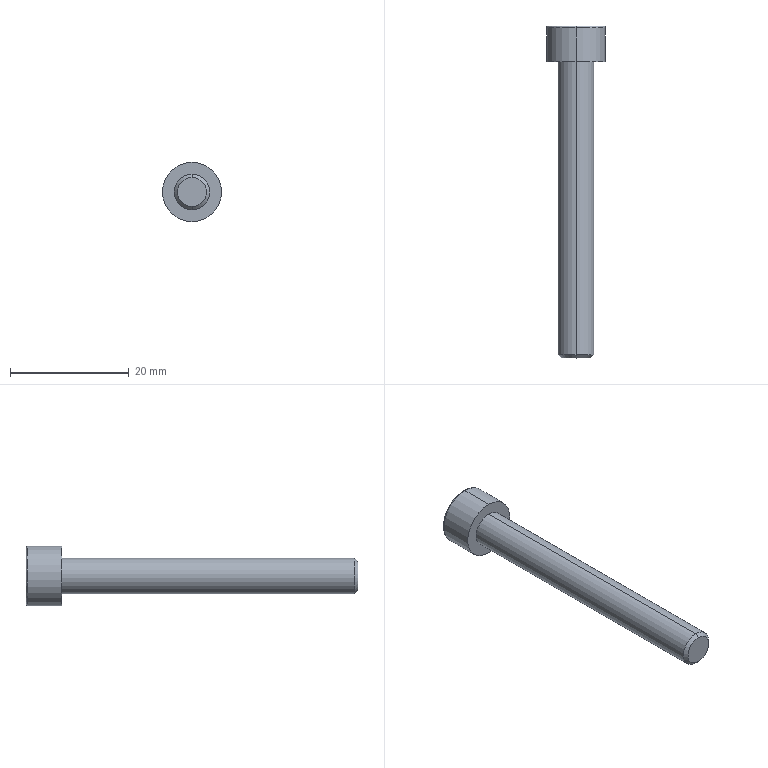Part | SolidWorks | features BaseBody 1 | 1 solid | 18 faces | box 10 x 56 x 10 mm | volume 1815 mm3 | plane 10 | cylinder 4 | cone 2 | torus 2 | commonest cylinder face diameters 6 x2 10 x2
STEP:
#1=CARTESIAN_POINT('',(0.,-50.,-2.445));
#2=VERTEX_POINT('',#1);
#3=CARTESIAN_POINT('',(0.,-50.,2.445));
#4=VERTEX_POINT('',#3);
#5=CARTESIAN_POINT('',(0.,-50.,0.));
#6=DIRECTION('',(0.,-1.,0.));
#7=DIRECTION('',(0.,0.,-1.));
#8=AXIS2_PLACEMENT_3D('',#5,#6,#7);
#9=CIRCLE('',#8,2.445);
#10=EDGE_CURVE('',#2,#4,#9,.T.);
#11=ORIENTED_EDGE('',*,*,#10,.F.);
#12=CARTESIAN_POINT('',(0.,-49.445,-3.));
#13=VERTEX_POINT('',#12);
#14=CARTESIAN_POINT('',(0.,-50.,-2.445));
#15=DIRECTION('',(0.,0.7071,-0.7071));
#16=VECTOR('',#15,1000.);
#17=LINE('',#14,#16);
#18=EDGE_CURVE('',#2,#13,#17,.T.);
#19=ORIENTED_EDGE('',*,*,#18,.T.);
#20=CARTESIAN_POINT('',(0.,-49.445,3.));
#21=VERTEX_POINT('',#20);
#22=CARTESIAN_POINT('',(0.,-49.445,0.));
#23=DIRECTION('',(0.,1.,0.));
#24=DIRECTION('',(0.,0.,-1.));
#25=AXIS2_PLACEMENT_3D('',#22,#23,#24);
#26=CIRCLE('',#25,3.);
#27=EDGE_CURVE('',#21,#13,#26,.T.);
#28=ORIENTED_EDGE('',*,*,#27,.F.);
#29=CARTESIAN_POINT('',(0.,-50.,2.445));
#30=DIRECTION('',(0.,0.7071,0.7071));
#31=VECTOR('',#30,1000.);
#32=LINE('',#29,#31);
#33=EDGE_CURVE('',#4,#21,#32,.T.);
#34=ORIENTED_EDGE('',*,*,#33,.F.);
#35=EDGE_LOOP('',(#11,#19,#28,#34));
#36=FACE_OUTER_BOUND('',#35,.T.);
#37=CARTESIAN_POINT('',(0.,-50.,0.));
#38=DIRECTION('',(0.,1.,0.));
#39=DIRECTION('',(0.,0.,1.));
#40=AXIS2_PLACEMENT_3D('',#37,#38,#39);
#41=CONICAL_SURFACE('',#40,2.445,0.7854);
#42=ADVANCED_FACE('',(#36),#41,.T.);
#43=ORIENTED_EDGE('',*,*,#27,.T.);
#44=CARTESIAN_POINT('',(0.,0.,-3.));
#45=VERTEX_POINT('',#44);
#46=CARTESIAN_POINT('',(0.,-50.,-3.));
#47=DIRECTION('',(0.,1.,0.));
#48=VECTOR('',#47,1000.);
#49=LINE('',#46,#48);
#50=EDGE_CURVE('',#13,#45,#49,.T.);
#51=ORIENTED_EDGE('',*,*,#50,.T.);
#52=CARTESIAN_POINT('',(0.,0.,3.));
#53=VERTEX_POINT('',#52);
#54=CARTESIAN_POINT('',(0.,0.,0.));
#55=DIRECTION('',(0.,-1.,0.));
#56=DIRECTION('',(0.,0.,1.));
#57=AXIS2_PLACEMENT_3D('',#54,#55,#56);
#58=CIRCLE('',#57,3.);
#59=EDGE_CURVE('',#45,#53,#58,.T.);
#60=ORIENTED_EDGE('',*,*,#59,.T.);
#61=CARTESIAN_POINT('',(0.,-50.,3.));
#62=DIRECTION('',(0.,1.,0.));
#63=VECTOR('',#62,1000.);
#64=LINE('',#61,#63);
#65=EDGE_CURVE('',#21,#53,#64,.T.);
#66=ORIENTED_EDGE('',*,*,#65,.F.);
#67=EDGE_LOOP('',(#43,#51,#60,#66));
#68=FACE_OUTER_BOUND('',#67,.T.);
#69=CARTESIAN_POINT('',(0.,-50.,0.));
#70=DIRECTION('',(0.,1.,0.));
#71=DIRECTION('',(0.,0.,1.));
#72=AXIS2_PLACEMENT_3D('',#69,#70,#71);
#73=CYLINDRICAL_SURFACE('',#72,3.);
#74=ADVANCED_FACE('',(#68),#73,.T.);
#75=CARTESIAN_POINT('',(0.,5.7,-5.));
#76=VERTEX_POINT('',#75);
#77=CARTESIAN_POINT('',(0.,5.7,5.));
#78=VERTEX_POINT('',#77);
#79=CARTESIAN_POINT('',(0.,5.7,0.));
#80=DIRECTION('',(0.,-1.,0.));
#81=DIRECTION('',(0.,0.,1.));
#82=AXIS2_PLACEMENT_3D('',#79,#80,#81);
#83=CIRCLE('',#82,5.);
#84=EDGE_CURVE('',#76,#78,#83,.T.);
#85=ORIENTED_EDGE('',*,*,#84,.F.);
#86=CARTESIAN_POINT('',(0.,6.,-4.7));
#87=VERTEX_POINT('',#86);
#88=CARTESIAN_POINT('',(0.,5.7,-4.7));
#89=DIRECTION('',(1.,0.,0.));
#90=DIRECTION('',(0.,0.,-1.));
#91=AXIS2_PLACEMENT_3D('',#88,#89,#90);
#92=CIRCLE('',#91,0.3);
#93=EDGE_CURVE('',#76,#87,#92,.T.);
#94=ORIENTED_EDGE('',*,*,#93,.T.);
#95=CARTESIAN_POINT('',(0.,6.,4.7));
#96=VERTEX_POINT('',#95);
#97=CARTESIAN_POINT('',(0.,6.,0.));
#98=DIRECTION('',(0.,1.,0.));
#99=DIRECTION('',(0.,0.,1.));
#100=AXIS2_PLACEMENT_3D('',#97,#98,#99);
#101=CIRCLE('',#100,4.7);
#102=EDGE_CURVE('',#96,#87,#101,.T.);
#103=ORIENTED_EDGE('',*,*,#102,.F.);
#104=CARTESIAN_POINT('',(0.,5.7,4.7));
#105=DIRECTION('',(-1.,0.,0.));
#106=DIRECTION('',(0.,0.,1.));
#107=AXIS2_PLACEMENT_3D('',#104,#105,#106);
#108=CIRCLE('',#107,0.3);
#109=EDGE_CURVE('',#78,#96,#108,.T.);
#110=ORIENTED_EDGE('',*,*,#109,.F.);
#111=EDGE_LOOP('',(#85,#94,#103,#110));
#112=FACE_OUTER_BOUND('',#111,.T.);
#113=CARTESIAN_POINT('',(0.,5.7,0.));
#114=DIRECTION('',(0.,1.,0.));
#115=DIRECTION('',(0.,0.,1.));
#116=AXIS2_PLACEMENT_3D('',#113,#114,#115);
#117=TOROIDAL_SURFACE('',#116,4.7,0.3);
#118=ADVANCED_FACE('',(#112),#117,.T.);
#119=ORIENTED_EDGE('',*,*,#84,.T.);
#120=CARTESIAN_POINT('',(0.,0.,5.));
#121=VERTEX_POINT('',#120);
#122=CARTESIAN_POINT('',(0.,6.,5.));
#123=DIRECTION('',(0.,-1.,0.));
#124=VECTOR('',#123,1000.);
#125=LINE('',#122,#124);
#126=EDGE_CURVE('',#78,#121,#125,.T.);
#127=ORIENTED_EDGE('',*,*,#126,.T.);
#128=CARTESIAN_POINT('',(0.,0.,-5.));
#129=VERTEX_POINT('',#128);
#130=CARTESIAN_POINT('',(0.,0.,0.));
#131=DIRECTION('',(0.,1.,0.));
#132=DIRECTION('',(0.,0.,1.));
#133=AXIS2_PLACEMENT_3D('',#130,#131,#132);
#134=CIRCLE('',#133,5.);
#135=EDGE_CURVE('',#121,#129,#134,.T.);
#136=ORIENTED_EDGE('',*,*,#135,.T.);
#137=CARTESIAN_POINT('',(0.,6.,-5.));
#138=DIRECTION('',(0.,-1.,0.));
#139=VECTOR('',#138,1000.);
#140=LINE('',#137,#139);
#141=EDGE_CURVE('',#76,#129,#140,.T.);
#142=ORIENTED_EDGE('',*,*,#141,.F.);
#143=EDGE_LOOP('',(#119,#127,#136,#142));
#144=FACE_OUTER_BOUND('',#143,.T.);
#145=CARTESIAN_POINT('',(0.,6.,0.));
#146=DIRECTION('',(0.,-1.,0.));
#147=DIRECTION('',(0.,0.,-1.));
#148=AXIS2_PLACEMENT_3D('',#145,#146,#147);
#149=CYLINDRICAL_SURFACE('',#148,5.);
#150=ADVANCED_FACE('',(#144),#149,.T.);
#151=CARTESIAN_POINT('',(0.,-50.,0.));
#152=DIRECTION('',(0.,-1.,0.));
#153=DIRECTION('',(0.,0.,-1.));
#154=AXIS2_PLACEMENT_3D('',#151,#152,#153);
#155=CIRCLE('',#154,2.445);
#156=EDGE_CURVE('',#4,#2,#155,.T.);
#157=ORIENTED_EDGE('',*,*,#156,.T.);
#158=ORIENTED_EDGE('',*,*,#10,.T.);
#159=EDGE_LOOP('',(#157,#158));
#160=FACE_OUTER_BOUND('',#159,.T.);
#161=CARTESIAN_POINT('',(0.,-50.,0.));
#162=DIRECTION('',(0.,-1.,0.));
#163=DIRECTION('',(0.,0.,-1.));
#164=AXIS2_PLACEMENT_3D('',#161,#162,#163);
#165=PLANE('',#164);
#166=ADVANCED_FACE('',(#160),#165,.T.);
#167=CARTESIAN_POINT('',(1.466,3.,2.54));
#168=VERTEX_POINT('',#167);
#169=CARTESIAN_POINT('',(2.933,3.,0.));
#170=VERTEX_POINT('',#169);
#171=CARTESIAN_POINT('',(1.466,3.,2.54));
#172=DIRECTION('',(0.5,0.,-0.866));
#173=VECTOR('',#172,1000.);
#174=LINE('',#171,#173);
#175=EDGE_CURVE('',#168,#170,#174,.T.);
#176=ORIENTED_EDGE('',*,*,#175,.T.);
#177=CARTESIAN_POINT('',(1.466,3.,-2.54));
#178=VERTEX_POINT('',#177);
#179=CARTESIAN_POINT('',(2.933,3.,0.));
#180=DIRECTION('',(-0.5,0.,-0.866));
#181=VECTOR('',#180,1000.);
#182=LINE('',#179,#181);
#183=EDGE_CURVE('',#170,#178,#182,.T.);
#184=ORIENTED_EDGE('',*,*,#183,.T.);
#185=CARTESIAN_POINT('',(-1.466,3.,-2.54));
#186=VERTEX_POINT('',#185);
#187=CARTESIAN_POINT('',(1.466,3.,-2.54));
#188=DIRECTION('',(-1.,0.,0.));
#189=VECTOR('',#188,1000.);
#190=LINE('',#187,#189);
#191=EDGE_CURVE('',#178,#186,#190,.T.);
#192=ORIENTED_EDGE('',*,*,#191,.T.);
#193=CARTESIAN_POINT('',(-2.933,3.,0.));
#194=VERTEX_POINT('',#193);
#195=CARTESIAN_POINT('',(-1.466,3.,-2.54));
#196=DIRECTION('',(-0.5,0.,0.866));
#197=VECTOR('',#196,1000.);
#198=LINE('',#195,#197);
#199=EDGE_CURVE('',#186,#194,#198,.T.);
#200=ORIENTED_EDGE('',*,*,#199,.T.);
#201=CARTESIAN_POINT('',(-1.466,3.,2.54));
#202=VERTEX_POINT('',#201);
#203=CARTESIAN_POINT('',(-2.933,3.,0.));
#204=DIRECTION('',(0.5,0.,0.866));
#205=VECTOR('',#204,1000.);
#206=LINE('',#203,#205);
#207=EDGE_CURVE('',#194,#202,#206,.T.);
#208=ORIENTED_EDGE('',*,*,#207,.T.);
#209=CARTESIAN_POINT('',(-1.466,3.,2.54));
#210=DIRECTION('',(1.,0.,0.));
#211=VECTOR('',#210,1000.);
#212=LINE('',#209,#211);
#213=EDGE_CURVE('',#202,#168,#212,.T.);
#214=ORIENTED_EDGE('',*,*,#213,.T.);
#215=EDGE_LOOP('',(#176,#184,#192,#200,#208,#214));
#216=FACE_OUTER_BOUND('',#215,.T.);
#217=CARTESIAN_POINT('',(0.,3.,0.));
#218=DIRECTION('',(0.,1.,0.));
#219=DIRECTION('',(1.,0.,0.));
#220=AXIS2_PLACEMENT_3D('',#217,#218,#219);
#221=PLANE('',#220);
#222=ADVANCED_FACE('',(#216),#221,.T.);
#223=CARTESIAN_POINT('',(2.933,6.,0.));
#224=VERTEX_POINT('',#223);
#225=CARTESIAN_POINT('',(1.466,6.,-2.54));
#226=VERTEX_POINT('',#225);
#227=CARTESIAN_POINT('',(2.933,6.,0.));
#228=DIRECTION('',(-0.5,0.,-0.866));
#229=VECTOR('',#228,1000.);
#230=LINE('',#227,#229);
#231=EDGE_CURVE('',#224,#226,#230,.T.);
#232=ORIENTED_EDGE('',*,*,#231,.T.);
#233=CARTESIAN_POINT('',(1.466,3.,-2.54));
#234=DIRECTION('',(0.,1.,0.));
#235=VECTOR('',#234,1000.);
#236=LINE('',#233,#235);
#237=EDGE_CURVE('',#178,#226,#236,.T.);
#238=ORIENTED_EDGE('',*,*,#237,.F.);
#239=ORIENTED_EDGE('',*,*,#183,.F.);
#240=CARTESIAN_POINT('',(2.933,3.,0.));
#241=DIRECTION('',(0.,1.,0.));
#242=VECTOR('',#241,1000.);
#243=LINE('',#240,#242);
#244=EDGE_CURVE('',#170,#224,#243,.T.);
#245=ORIENTED_EDGE('',*,*,#244,.T.);
#246=EDGE_LOOP('',(#232,#238,#239,#245));
#247=FACE_OUTER_BOUND('',#246,.T.);
#248=CARTESIAN_POINT('',(2.933,3.,0.));
#249=DIRECTION('',(0.866,0.,-0.5));
#250=DIRECTION('',(0.,-1.,0.));
#251=AXIS2_PLACEMENT_3D('',#248,#249,#250);
#252=PLANE('',#251);
#253=ADVANCED_FACE('',(#247),#252,.F.);
#254=CARTESIAN_POINT('',(-1.466,6.,-2.54));
#255=VERTEX_POINT('',#254);
#256=CARTESIAN_POINT('',(1.466,6.,-2.54));
#257=DIRECTION('',(-1.,0.,0.));
#258=VECTOR('',#257,1000.);
#259=LINE('',#256,#258);
#260=EDGE_CURVE('',#226,#255,#259,.T.);
#261=ORIENTED_EDGE('',*,*,#260,.T.);
#262=CARTESIAN_POINT('',(-1.466,3.,-2.54));
#263=DIRECTION('',(0.,1.,0.));
#264=VECTOR('',#263,1000.);
#265=LINE('',#262,#264);
#266=EDGE_CURVE('',#186,#255,#265,.T.);
#267=ORIENTED_EDGE('',*,*,#266,.F.);
#268=ORIENTED_EDGE('',*,*,#191,.F.);
#269=ORIENTED_EDGE('',*,*,#237,.T.);
#270=EDGE_LOOP('',(#261,#267,#268,#269));
#271=FACE_OUTER_BOUND('',#270,.T.);
#272=CARTESIAN_POINT('',(1.466,3.,-2.54));
#273=DIRECTION('',(0.,0.,-1.));
#274=DIRECTION('',(0.,-1.,0.));
#275=AXIS2_PLACEMENT_3D('',#272,#273,#274);
#276=PLANE('',#275);
#277=ADVANCED_FACE('',(#271),#276,.F.);
#278=CARTESIAN_POINT('',(-2.933,6.,0.));
#279=VERTEX_POINT('',#278);
#280=CARTESIAN_POINT('',(-1.466,6.,-2.54));
#281=DIRECTION('',(-0.5,0.,0.866));
#282=VECTOR('',#281,1000.);
#283=LINE('',#280,#282);
#284=EDGE_CURVE('',#255,#279,#283,.T.);
#285=ORIENTED_EDGE('',*,*,#284,.T.);
#286=CARTESIAN_POINT('',(-2.933,3.,0.));
#287=DIRECTION('',(0.,1.,0.));
#288=VECTOR('',#287,1000.);
#289=LINE('',#286,#288);
#290=EDGE_CURVE('',#194,#279,#289,.T.);
#291=ORIENTED_EDGE('',*,*,#290,.F.);
#292=ORIENTED_EDGE('',*,*,#199,.F.);
#293=ORIENTED_EDGE('',*,*,#266,.T.);
#294=EDGE_LOOP('',(#285,#291,#292,#293));
#295=FACE_OUTER_BOUND('',#294,.T.);
#296=CARTESIAN_POINT('',(-1.466,3.,-2.54));
#297=DIRECTION('',(-0.866,0.,-0.5));
#298=DIRECTION('',(-0.5,0.,0.866));
#299=AXIS2_PLACEMENT_3D('',#296,#297,#298);
#300=PLANE('',#299);
#301=ADVANCED_FACE('',(#295),#300,.F.);
#302=CARTESIAN_POINT('',(-1.466,6.,2.54));
#303=VERTEX_POINT('',#302);
#304=CARTESIAN_POINT('',(-2.933,6.,0.));
#305=DIRECTION('',(0.5,0.,0.866));
#306=VECTOR('',#305,1000.);
#307=LINE('',#304,#306);
#308=EDGE_CURVE('',#279,#303,#307,.T.);
#309=ORIENTED_EDGE('',*,*,#308,.T.);
#310=CARTESIAN_POINT('',(-1.466,3.,2.54));
#311=DIRECTION('',(0.,1.,0.));
#312=VECTOR('',#311,1000.);
#313=LINE('',#310,#312);
#314=EDGE_CURVE('',#202,#303,#313,.T.);
#315=ORIENTED_EDGE('',*,*,#314,.F.);
#316=ORIENTED_EDGE('',*,*,#207,.F.);
#317=ORIENTED_EDGE('',*,*,#290,.T.);
#318=EDGE_LOOP('',(#309,#315,#316,#317));
#319=FACE_OUTER_BOUND('',#318,.T.);
#320=CARTESIAN_POINT('',(-2.933,3.,0.));
#321=DIRECTION('',(-0.866,0.,0.5));
#322=DIRECTION('',(0.,1.,0.));
#323=AXIS2_PLACEMENT_3D('',#320,#321,#322);
#324=PLANE('',#323);
#325=ADVANCED_FACE('',(#319),#324,.F.);
#326=CARTESIAN_POINT('',(1.466,6.,2.54));
#327=VERTEX_POINT('',#326);
#328=CARTESIAN_POINT('',(-1.466,6.,2.54));
#329=DIRECTION('',(1.,0.,0.));
#330=VECTOR('',#329,1000.);
#331=LINE('',#328,#330);
#332=EDGE_CURVE('',#303,#327,#331,.T.);
#333=ORIENTED_EDGE('',*,*,#332,.T.);
#334=CARTESIAN_POINT('',(1.466,3.,2.54));
#335=DIRECTION('',(0.,1.,0.));
#336=VECTOR('',#335,1000.);
#337=LINE('',#334,#336);
#338=EDGE_CURVE('',#168,#327,#337,.T.);
#339=ORIENTED_EDGE('',*,*,#338,.F.);
#340=ORIENTED_EDGE('',*,*,#213,.F.);
#341=ORIENTED_EDGE('',*,*,#314,.T.);
#342=EDGE_LOOP('',(#333,#339,#340,#341));
#343=FACE_OUTER_BOUND('',#342,.T.);
#344=CARTESIAN_POINT('',(-1.466,3.,2.54));
#345=DIRECTION('',(0.,0.,1.));
#346=DIRECTION('',(1.,0.,0.));
#347=AXIS2_PLACEMENT_3D('',#344,#345,#346);
#348=PLANE('',#347);
#349=ADVANCED_FACE('',(#343),#348,.F.);
#350=CARTESIAN_POINT('',(1.466,6.,2.54));
#351=DIRECTION('',(0.5,0.,-0.866));
#352=VECTOR('',#351,1000.);
#353=LINE('',#350,#352);
#354=EDGE_CURVE('',#327,#224,#353,.T.);
#355=ORIENTED_EDGE('',*,*,#354,.T.);
#356=ORIENTED_EDGE('',*,*,#244,.F.);
#357=ORIENTED_EDGE('',*,*,#175,.F.);
#358=ORIENTED_EDGE('',*,*,#338,.T.);
#359=EDGE_LOOP('',(#355,#356,#357,#358));
#360=FACE_OUTER_BOUND('',#359,.T.);
#361=CARTESIAN_POINT('',(1.466,3.,2.54));
#362=DIRECTION('',(0.866,0.,0.5));
#363=DIRECTION('',(0.,-1.,0.));
#364=AXIS2_PLACEMENT_3D('',#361,#362,#363);
#365=PLANE('',#364);
#366=ADVANCED_FACE('',(#360),#365,.F.);
#367=ORIENTED_EDGE('',*,*,#354,.F.);
#368=ORIENTED_EDGE('',*,*,#332,.F.);
#369=ORIENTED_EDGE('',*,*,#308,.F.);
#370=ORIENTED_EDGE('',*,*,#284,.F.);
#371=ORIENTED_EDGE('',*,*,#260,.F.);
#372=ORIENTED_EDGE('',*,*,#231,.F.);
#373=EDGE_LOOP('',(#367,#368,#369,#370,#371,#372));
#374=FACE_BOUND('',#373,.T.);
#375=ORIENTED_EDGE('',*,*,#102,.T.);
#376=CARTESIAN_POINT('',(0.,6.,0.));
#377=DIRECTION('',(0.,1.,0.));
#378=DIRECTION('',(0.,0.,1.));
#379=AXIS2_PLACEMENT_3D('',#376,#377,#378);
#380=CIRCLE('',#379,4.7);
#381=EDGE_CURVE('',#87,#96,#380,.T.);
#382=ORIENTED_EDGE('',*,*,#381,.T.);
#383=EDGE_LOOP('',(#375,#382));
#384=FACE_OUTER_BOUND('',#383,.T.);
#385=CARTESIAN_POINT('',(0.,6.,0.));
#386=DIRECTION('',(0.,1.,0.));
#387=DIRECTION('',(1.,0.,0.));
#388=AXIS2_PLACEMENT_3D('',#385,#386,#387);
#389=PLANE('',#388);
#390=ADVANCED_FACE('',(#374,#384),#389,.T.);
#391=CARTESIAN_POINT('',(0.,0.,0.));
#392=DIRECTION('',(0.,-1.,0.));
#393=DIRECTION('',(0.,0.,1.));
#394=AXIS2_PLACEMENT_3D('',#391,#392,#393);
#395=CIRCLE('',#394,3.);
#396=EDGE_CURVE('',#53,#45,#395,.T.);
#397=ORIENTED_EDGE('',*,*,#396,.F.);
#398=ORIENTED_EDGE('',*,*,#59,.F.);
#399=EDGE_LOOP('',(#397,#398));
#400=FACE_BOUND('',#399,.T.);
#401=CARTESIAN_POINT('',(0.,0.,0.));
#402=DIRECTION('',(0.,1.,0.));
#403=DIRECTION('',(0.,0.,1.));
#404=AXIS2_PLACEMENT_3D('',#401,#402,#403);
#405=CIRCLE('',#404,5.);
#406=EDGE_CURVE('',#129,#121,#405,.T.);
#407=ORIENTED_EDGE('',*,*,#406,.F.);
#408=ORIENTED_EDGE('',*,*,#135,.F.);
#409=EDGE_LOOP('',(#407,#408));
#410=FACE_OUTER_BOUND('',#409,.T.);
#411=CARTESIAN_POINT('',(0.,0.,0.));
#412=DIRECTION('',(0.,1.,0.));
#413=DIRECTION('',(1.,0.,0.));
#414=AXIS2_PLACEMENT_3D('',#411,#412,#413);
#415=PLANE('',#414);
#416=ADVANCED_FACE('',(#400,#410),#415,.F.);
#417=ORIENTED_EDGE('',*,*,#126,.F.);
#418=CARTESIAN_POINT('',(0.,5.7,0.));
#419=DIRECTION('',(0.,-1.,0.));
#420=DIRECTION('',(0.,0.,1.));
#421=AXIS2_PLACEMENT_3D('',#418,#419,#420);
#422=CIRCLE('',#421,5.);
#423=EDGE_CURVE('',#78,#76,#422,.T.);
#424=ORIENTED_EDGE('',*,*,#423,.T.);
#425=ORIENTED_EDGE('',*,*,#141,.T.);
#426=ORIENTED_EDGE('',*,*,#406,.T.);
#427=EDGE_LOOP('',(#417,#424,#425,#426));
#428=FACE_OUTER_BOUND('',#427,.T.);
#429=CARTESIAN_POINT('',(0.,6.,0.));
#430=DIRECTION('',(0.,-1.,0.));
#431=DIRECTION('',(0.,0.,-1.));
#432=AXIS2_PLACEMENT_3D('',#429,#430,#431);
#433=CYLINDRICAL_SURFACE('',#432,5.);
#434=ADVANCED_FACE('',(#428),#433,.T.);
#435=ORIENTED_EDGE('',*,*,#93,.F.);
#436=ORIENTED_EDGE('',*,*,#423,.F.);
#437=ORIENTED_EDGE('',*,*,#109,.T.);
#438=ORIENTED_EDGE('',*,*,#381,.F.);
#439=EDGE_LOOP('',(#435,#436,#437,#438));
#440=FACE_OUTER_BOUND('',#439,.T.);
#441=CARTESIAN_POINT('',(0.,5.7,0.));
#442=DIRECTION('',(0.,1.,0.));
#443=DIRECTION('',(0.,0.,1.));
#444=AXIS2_PLACEMENT_3D('',#441,#442,#443);
#445=TOROIDAL_SURFACE('',#444,4.7,0.3);
#446=ADVANCED_FACE('',(#440),#445,.T.);
#447=ORIENTED_EDGE('',*,*,#50,.F.);
#448=CARTESIAN_POINT('',(0.,-49.445,0.));
#449=DIRECTION('',(0.,1.,0.));
#450=DIRECTION('',(0.,0.,-1.));
#451=AXIS2_PLACEMENT_3D('',#448,#449,#450);
#452=CIRCLE('',#451,3.);
#453=EDGE_CURVE('',#13,#21,#452,.T.);
#454=ORIENTED_EDGE('',*,*,#453,.T.);
#455=ORIENTED_EDGE('',*,*,#65,.T.);
#456=ORIENTED_EDGE('',*,*,#396,.T.);
#457=EDGE_LOOP('',(#447,#454,#455,#456));
#458=FACE_OUTER_BOUND('',#457,.T.);
#459=CARTESIAN_POINT('',(0.,-50.,0.));
#460=DIRECTION('',(0.,1.,0.));
#461=DIRECTION('',(0.,0.,1.));
#462=AXIS2_PLACEMENT_3D('',#459,#460,#461);
#463=CYLINDRICAL_SURFACE('',#462,3.);
#464=ADVANCED_FACE('',(#458),#463,.T.);
#465=ORIENTED_EDGE('',*,*,#18,.F.);
#466=ORIENTED_EDGE('',*,*,#156,.F.);
#467=ORIENTED_EDGE('',*,*,#33,.T.);
#468=ORIENTED_EDGE('',*,*,#453,.F.);
#469=EDGE_LOOP('',(#465,#466,#467,#468));
#470=FACE_OUTER_BOUND('',#469,.T.);
#471=CARTESIAN_POINT('',(0.,-50.,0.));
#472=DIRECTION('',(0.,1.,0.));
#473=DIRECTION('',(0.,0.,1.));
#474=AXIS2_PLACEMENT_3D('',#471,#472,#473);
#475=CONICAL_SURFACE('',#474,2.445,0.7854);
#476=ADVANCED_FACE('',(#470),#475,.T.);
#477=CLOSED_SHELL('',(#42,#74,#118,#150,#166,#222,#253,#277,#301,#325,#349,#366,#390,#416,#434,#446,#464,#476));
#478=MANIFOLD_SOLID_BREP('',#477);
#479=CARTESIAN_POINT('',(0.,0.,0.));
#480=DIRECTION('',(0.,0.,1.));
#481=DIRECTION('',(1.,0.,0.));
#482=AXIS2_PLACEMENT_3D('',#479,#480,#481);
#483=(LENGTH_UNIT()NAMED_UNIT(*)SI_UNIT(.MILLI.,.METRE.));
#484=UNCERTAINTY_MEASURE_WITH_UNIT(LENGTH_MEASURE(0.00001),#483,'','');
#485=(NAMED_UNIT(*)PLANE_ANGLE_UNIT()SI_UNIT($,.RADIAN.));
#486=(NAMED_UNIT(*)SI_UNIT($,.STERADIAN.)SOLID_ANGLE_UNIT());
#487=(GEOMETRIC_REPRESENTATION_CONTEXT(3)GLOBAL_UNCERTAINTY_ASSIGNED_CONTEXT((#484))GLOBAL_UNIT_ASSIGNED_CONTEXT((#483,#485,#486))REPRESENTATION_CONTEXT('',''));
#488=ADVANCED_BREP_SHAPE_REPRESENTATION('',(#478,#482),#487);